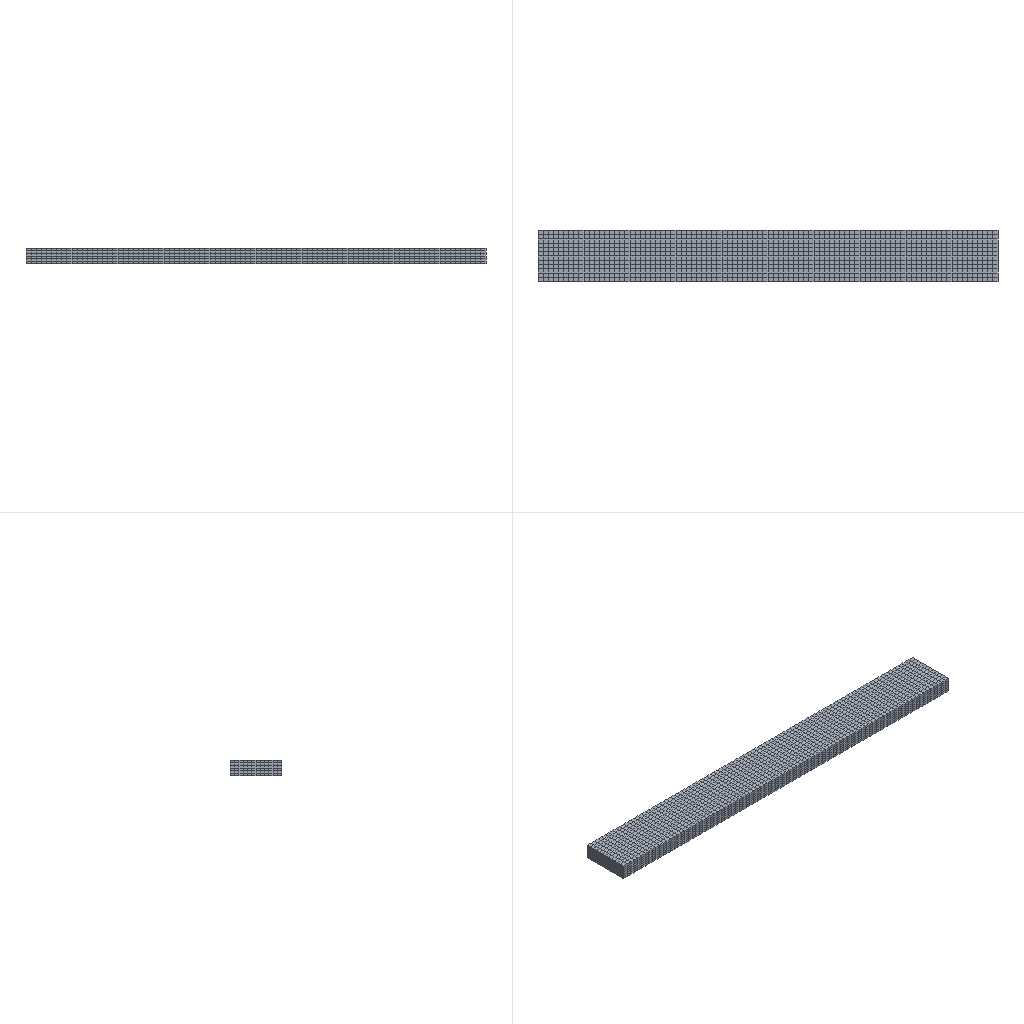Simulation study | abaqus
Set-up summary:
category,name,step,type,value,unit,region
solver,abaqus
solver,version,,,Abaqus/Standard 3DEXPERIENCE R2017x
units,not stated in the deck,,not stated
analysis,deck,,static,static
load_step,Step-1,Step-1,static,nlgeom=False
contact,interactions,,,general=0 pairs=0 ties=0
load_step,requested,,,1
mesh,nodes,,,8281
mesh,elements,,,6480
element_type,C3D8R,,solid,6480
load,load commands in deck,,count,1
bc,support commands in deck,,count,7
material,MATERIAL-1,,in results
check,setup vs results,,match,"per instance, exact: element labels, types and connectivity; labels of the nodes the elements use; coordinates of those nodes at SINGLE_PRECISION in 1 of 1 instance(s)"
Abaqus input file, long lists of numbers shortened:
*Heading
** Job name: Job-3 Model name: Model-3
** Generated by: Abaqus/CAE 2017
*Preprint, echo=NO, model=NO, history=NO, contact=NO
**
** PARTS
**
*Part, name=Part-1
*Node
      1,          15.,          2.5,           2.
      2,          20.,          2.5,           2.
** (8279 more lines like these left out)
*Element, type=C3D8R
 1,  406, 2734, 6554, 2730,    1,  381, 2714,  392
 2, 2734, 2735, 6555, 6554,  381,  382, 2715, 2714
** (6478 more lines like these left out)
*Nset, nset=Set-1, generate
    1,  8281,     1
*Elset, elset=Set-1, generate
    1,  6480,     1
** Section: Section-1
*Solid Section, elset=Set-1, material=Material-1
,
*End Part
**
**
** ASSEMBLY
**
*Assembly, name=Assembly
**
*Instance, name=Part-1-1, part=Part-1
*End Instance
**
*Node
      1,          90.,           5.,          1.5
*Nset, nset=Set-8, instance=Part-1-1, generate
    1,  8281,     1
*Elset, elset=Set-8, instance=Part-1-1, generate
    1,  6480,     1
*Nset, nset=Set-9, instance=Part-1-1
  286,  287,  288,  289,  290,  291,  292,  293,  294,  295,  296,  297,  298,  299,  300,  301
  302,  303,  304,  305,  306,  307,  308,  309,  310,  311,  312,  313,  314,  315,  316,  317
** (72 more lines like these left out)
*Elset, elset=Set-9, instance=Part-1-1
 4306, 4307, 4308, 4309, 4310, 4311, 4312, 4313, 4314, 4315, 4316, 4317, 4318, 4319, 4320, 4336
 4337, 4338, 4339, 4340, 4341, 4342, 4343, 4344, 4345, 4346, 4347, 4348, 4349, 4350, 4366, 4367
** (66 more lines like these left out)
*Nset, nset=Set-10, instance=Part-1-1, generate
    1,  8281,     1
*Elset, elset=Set-10, instance=Part-1-1, generate
    1,  6480,     1
*Nset, nset=Set-11, instance=Part-1-1
  175,  176,  177,  178,  179,  180,  182,  184,  188,  190,  278,  279,  280,  282,  285,  352
  353,  354,  355,  356, 1408, 1409, 1418, 1419, 1420, 1421, 1426, 1427, 1432, 1433, 1434, 1437
** (4 more lines like these left out)
*Elset, elset=Set-11, instance=Part-1-1
 1921, 1926, 1931, 1936, 1941, 1946, 1951, 1956, 1961, 1966, 1971, 1976, 1993, 1994, 1995, 2008
 2009, 2010, 2083, 2084, 2085, 2098, 2099, 2100, 4051, 4056, 4061, 4066, 4071, 4076, 4081, 4086
** (3 more lines like these left out)
*Nset, nset=Set-13
 1,
*Nset, nset=Set-217, instance=Part-1-1, generate
    1,  8281,     1
*Elset, elset=Set-217, instance=Part-1-1, generate
    1,  6480,     1
*Nset, nset=Set-218, instance=Part-1-1, generate
    1,  8281,     1
*Elset, elset=Set-218, instance=Part-1-1, generate
    1,  6480,     1
*Nset, nset=Set-219, instance=Part-1-1, generate
    1,  8281,     1
*Elset, elset=Set-219, instance=Part-1-1, generate
    1,  6480,     1
*Nset, nset=Set-220, instance=Part-1-1
  286,  287,  288,  289,  290,  291,  292,  293,  294,  295,  296,  297,  298,  299,  300,  301
  302,  303,  304,  305,  306,  307,  308,  309,  310,  311,  312,  313,  314,  315,  316,  317
** (72 more lines like these left out)
*Elset, elset=Set-220, instance=Part-1-1
 4306, 4307, 4308, 4309, 4310, 4311, 4312, 4313, 4314, 4315, 4316, 4317, 4318, 4319, 4320, 4336
 4337, 4338, 4339, 4340, 4341, 4342, 4343, 4344, 4345, 4346, 4347, 4348, 4349, 4350, 4366, 4367
** (66 more lines like these left out)
*Nset, nset=Set-221, instance=Part-1-1, generate
    1,  8281,     1
*Elset, elset=Set-221, instance=Part-1-1, generate
    1,  6480,     1
*Nset, nset=Set-222, instance=Part-1-1, generate
    1,  8281,     1
*Elset, elset=Set-222, instance=Part-1-1, generate
    1,  6480,     1
*Nset, nset=Set-223, instance=Part-1-1, generate
    1,  8281,     1
*Elset, elset=Set-223, instance=Part-1-1, generate
    1,  6480,     1
*Nset, nset=m_Set-12
 1,
*Elset, elset=_s_Surf-1_S5, internal, instance=Part-1-1
 1423, 1424, 1425, 1438, 1439, 1440, 3553, 3554, 3555, 3568, 3569, 3570, 6253, 6254, 6255, 6268
 6269, 6270
*Elset, elset=_s_Surf-1_S6, internal, instance=Part-1-1
 1321, 1326, 1331, 1336, 1341, 1346, 1351, 1356, 1361, 1366, 1371, 1376, 1381, 1386, 1391, 1396
 1401, 1406, 3451, 3456, 3461, 3466, 3471, 3476, 3481, 3486, 3491, 3496, 3501, 3506, 3511, 3516
** (1 more lines like these left out)
*Elset, elset=_s_Surf-1_S3, internal, instance=Part-1-1
 6331, 6332, 6333, 6346, 6347, 6348
*Elset, elset=_s_Surf-1_S4, internal, instance=Part-1-1, generate
 6395,  6420,     5
*Surface, type=ELEMENT, name=s_Surf-1
_s_Surf-1_S5, S5
_s_Surf-1_S6, S6
_s_Surf-1_S4, S4
_s_Surf-1_S3, S3
** Constraint: Constraint-1
*Coupling, constraint name=Constraint-1, ref node=m_Set-12, surface=s_Surf-1
*Kinematic
*End Assembly
*Amplitude, name=Amp-1
             0.,              0.,              1.,              1.
**
** MATERIALS
**
*Material, name=Material-1
*Density
 2.7e-09,
*Elastic
12500., 0.35
*Expansion
 1e-06,
** ----------------------------------------------------------------
**
** STEP: Step-1
**
*Step, name=Step-1, nlgeom=NO, inc=1000
*Static, stabilize=0.0002, allsdtol=0.05, continue=NO
0.01, 1., 1e-05, 0.1
**
** BOUNDARY CONDITIONS
**
** Name: BC-2 Type: 对称/反对称/完全固定
*Boundary
Set-11, ENCASTRE
** Name: [REDACTED] : Displacement/rotation angle
*Boundary, amplitude=Amp-1
Set-13, 1, 1, 5.
Set-13, 2, 2
Set-13, 3, 3
Set-13, 4, 4
Set-13, 5, 5
Set-13, 6, 6
**
** OUTPUT REQUESTS
**
*Restart, write, frequency=0
**
** FIELD OUTPUT: F-Output-1
**
*Output, field, variable=PRESELECT
**
** HISTORY OUTPUT: H-Output-1
**
*Output, history, variable=PRESELECT
*End Step
Results summary:
result,step,,completed,increments=15 time=1.0/1.0
result,analysis,,,static
result,last_loadstep,,,1
result,analysis steps,,count,1
result,primary field,,,U
result,reaction total,,FX,0.1597,model units
result,reaction total,,FY,1.1e-05,model units
result,reaction total,,FZ,-0.0,model units